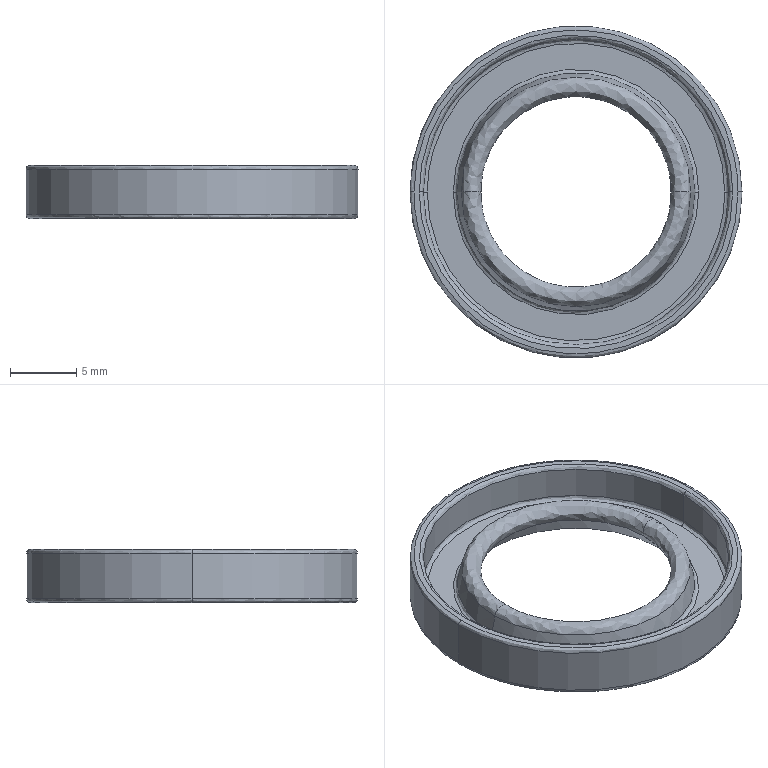Part | STEP file | 31740004--1-SOLI00_1_1_1 | 1 solid | 25 faces | box 25 x 25 x 4 mm | volume 623.091 mm3 | spline 14 | cone 4 | cylinder 4 | plane 3 | commonest cylinder face diameters 23 x2 25 x2